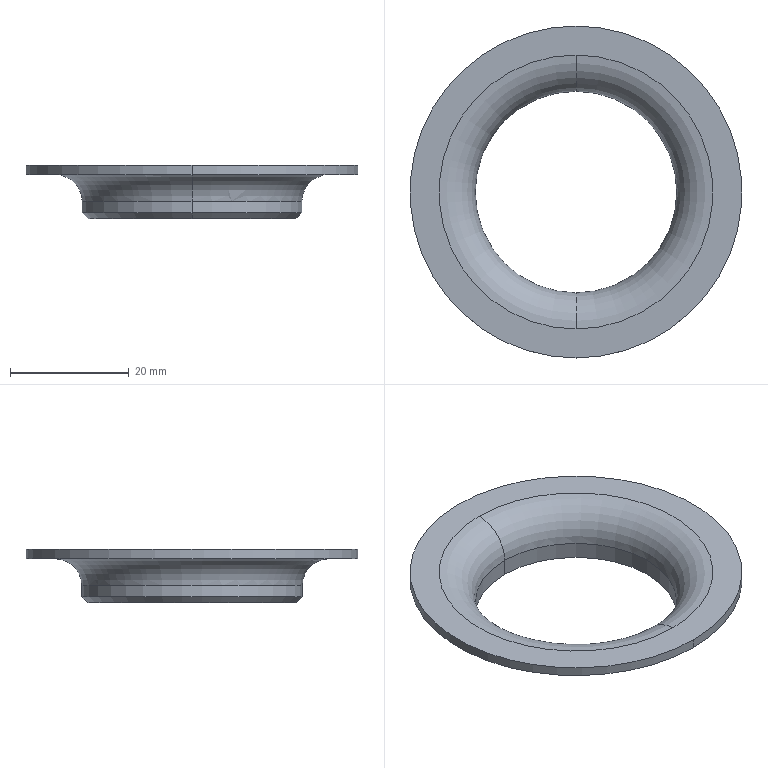Part | STEP file | YLG_9_1_1_1 | 1 solid | 15 faces | box 56 x 56 x 9 mm | volume 3369 mm3 | cylinder 6 | torus 4 | plane 3 | cone 2 | commonest cylinder face diameters 34 x2 37.2 x2 56 x2
STEP:
#1=CARTESIAN_POINT('',(0.,0.,0.));
#2=DIRECTION('',(0.,0.,1.));
#3=DIRECTION('',(1.,0.,0.));
#4=AXIS2_PLACEMENT_3D('',#1,#2,#3);
#5=CARTESIAN_POINT('',(0.,-17.,-10.));
#6=VERTEX_POINT('',#5);
#7=CARTESIAN_POINT('',(0.,-23.1,-3.9));
#8=VERTEX_POINT('',#7);
#9=CARTESIAN_POINT('',(0.,-23.1,-10.));
#10=DIRECTION('',(1.,0.,0.));
#11=DIRECTION('',(0.,1.,0.));
#12=AXIS2_PLACEMENT_3D('',#9,#10,#11);
#13=CIRCLE('',#12,6.1);
#14=EDGE_CURVE('',#6,#8,#13,.T.);
#15=ORIENTED_EDGE('',*,*,#14,.F.);
#16=CARTESIAN_POINT('',(0.,17.,-10.));
#17=VERTEX_POINT('',#16);
#18=CARTESIAN_POINT('',(0.,0.,-10.));
#19=DIRECTION('',(0.,0.,1.));
#20=DIRECTION('',(0.,-1.,0.));
#21=AXIS2_PLACEMENT_3D('',#18,#19,#20);
#22=CIRCLE('',#21,17.);
#23=EDGE_CURVE('',#6,#17,#22,.T.);
#24=ORIENTED_EDGE('',*,*,#23,.T.);
#25=CARTESIAN_POINT('',(0.,23.1,-3.9));
#26=VERTEX_POINT('',#25);
#27=CARTESIAN_POINT('',(0.,23.1,-10.));
#28=DIRECTION('',(-1.,0.,0.));
#29=DIRECTION('',(0.,-1.,0.));
#30=AXIS2_PLACEMENT_3D('',#27,#28,#29);
#31=CIRCLE('',#30,6.1);
#32=EDGE_CURVE('',#17,#26,#31,.T.);
#33=ORIENTED_EDGE('',*,*,#32,.T.);
#34=CARTESIAN_POINT('',(0.,0.,-3.9));
#35=DIRECTION('',(0.,0.,1.));
#36=DIRECTION('',(0.,-1.,0.));
#37=AXIS2_PLACEMENT_3D('',#34,#35,#36);
#38=CIRCLE('',#37,23.1);
#39=EDGE_CURVE('',#8,#26,#38,.T.);
#40=ORIENTED_EDGE('',*,*,#39,.F.);
#41=EDGE_LOOP('',(#15,#24,#33,#40));
#42=FACE_OUTER_BOUND('',#41,.F.);
#43=CARTESIAN_POINT('',(0.,0.,-10.));
#44=DIRECTION('',(0.,0.,1.));
#45=DIRECTION('',(0.,1.,0.));
#46=AXIS2_PLACEMENT_3D('',#43,#44,#45);
#47=TOROIDAL_SURFACE('',#46,23.1,6.1);
#48=ADVANCED_FACE('',(#42),#47,.T.);
#49=ORIENTED_EDGE('',*,*,#14,.T.);
#50=CARTESIAN_POINT('',(0.,0.,-3.9));
#51=DIRECTION('',(0.,0.,1.));
#52=DIRECTION('',(0.,1.,0.));
#53=AXIS2_PLACEMENT_3D('',#50,#51,#52);
#54=CIRCLE('',#53,23.1);
#55=EDGE_CURVE('',#26,#8,#54,.T.);
#56=ORIENTED_EDGE('',*,*,#55,.F.);
#57=ORIENTED_EDGE('',*,*,#32,.F.);
#58=CARTESIAN_POINT('',(0.,0.,-10.));
#59=DIRECTION('',(0.,0.,1.));
#60=DIRECTION('',(0.,1.,0.));
#61=AXIS2_PLACEMENT_3D('',#58,#59,#60);
#62=CIRCLE('',#61,17.);
#63=EDGE_CURVE('',#17,#6,#62,.T.);
#64=ORIENTED_EDGE('',*,*,#63,.T.);
#65=EDGE_LOOP('',(#49,#56,#57,#64));
#66=FACE_OUTER_BOUND('',#65,.F.);
#67=CARTESIAN_POINT('',(0.,0.,-10.));
#68=DIRECTION('',(0.,0.,1.));
#69=DIRECTION('',(0.,1.,0.));
#70=AXIS2_PLACEMENT_3D('',#67,#68,#69);
#71=TOROIDAL_SURFACE('',#70,23.1,6.1);
#72=ADVANCED_FACE('',(#66),#71,.T.);
#73=CARTESIAN_POINT('',(0.,28.,-3.9));
#74=VERTEX_POINT('',#73);
#75=CARTESIAN_POINT('',(0.,-28.,-3.9));
#76=VERTEX_POINT('',#75);
#77=CARTESIAN_POINT('',(0.,0.,-3.9));
#78=DIRECTION('',(0.,0.,-1.));
#79=DIRECTION('',(0.,1.,0.));
#80=AXIS2_PLACEMENT_3D('',#77,#78,#79);
#81=CIRCLE('',#80,28.);
#82=EDGE_CURVE('',#74,#76,#81,.T.);
#83=ORIENTED_EDGE('',*,*,#82,.T.);
#84=CARTESIAN_POINT('',(0.,0.,-3.9));
#85=DIRECTION('',(0.,0.,-1.));
#86=DIRECTION('',(0.,-1.,0.));
#87=AXIS2_PLACEMENT_3D('',#84,#85,#86);
#88=CIRCLE('',#87,28.);
#89=EDGE_CURVE('',#76,#74,#88,.T.);
#90=ORIENTED_EDGE('',*,*,#89,.T.);
#91=EDGE_LOOP('',(#83,#90));
#92=FACE_OUTER_BOUND('',#91,.F.);
#93=ORIENTED_EDGE('',*,*,#55,.T.);
#94=ORIENTED_EDGE('',*,*,#39,.T.);
#95=EDGE_LOOP('',(#93,#94));
#96=FACE_BOUND('',#95,.F.);
#97=CARTESIAN_POINT('',(0.,0.,-3.9));
#98=DIRECTION('',(0.,0.,1.));
#99=DIRECTION('',(0.,1.,0.));
#100=AXIS2_PLACEMENT_3D('',#97,#98,#99);
#101=PLANE('',#100);
#102=ADVANCED_FACE('',(#92,#96),#101,.T.);
#103=CARTESIAN_POINT('',(0.,-28.,-5.5));
#104=VERTEX_POINT('',#103);
#105=CARTESIAN_POINT('',(0.,-28.,-3.9));
#106=DIRECTION('',(0.,0.,-1.));
#107=VECTOR('',#106,1.6);
#108=LINE('',#105,#107);
#109=EDGE_CURVE('',#76,#104,#108,.T.);
#110=ORIENTED_EDGE('',*,*,#109,.F.);
#111=ORIENTED_EDGE('',*,*,#82,.F.);
#112=CARTESIAN_POINT('',(0.,28.,-5.5));
#113=VERTEX_POINT('',#112);
#114=CARTESIAN_POINT('',(0.,28.,-3.9));
#115=DIRECTION('',(0.,0.,-1.));
#116=VECTOR('',#115,1.6);
#117=LINE('',#114,#116);
#118=EDGE_CURVE('',#74,#113,#117,.T.);
#119=ORIENTED_EDGE('',*,*,#118,.T.);
#120=CARTESIAN_POINT('',(0.,0.,-5.5));
#121=DIRECTION('',(0.,0.,1.));
#122=DIRECTION('',(0.,-1.,0.));
#123=AXIS2_PLACEMENT_3D('',#120,#121,#122);
#124=CIRCLE('',#123,28.);
#125=EDGE_CURVE('',#104,#113,#124,.T.);
#126=ORIENTED_EDGE('',*,*,#125,.F.);
#127=EDGE_LOOP('',(#110,#111,#119,#126));
#128=FACE_OUTER_BOUND('',#127,.F.);
#129=CARTESIAN_POINT('',(0.,0.,0.));
#130=DIRECTION('',(0.,0.,1.));
#131=DIRECTION('',(0.,1.,0.));
#132=AXIS2_PLACEMENT_3D('',#129,#130,#131);
#133=CYLINDRICAL_SURFACE('',#132,28.);
#134=ADVANCED_FACE('',(#128),#133,.T.);
#135=ORIENTED_EDGE('',*,*,#109,.T.);
#136=CARTESIAN_POINT('',(0.,0.,-5.5));
#137=DIRECTION('',(0.,0.,1.));
#138=DIRECTION('',(0.,1.,0.));
#139=AXIS2_PLACEMENT_3D('',#136,#137,#138);
#140=CIRCLE('',#139,28.);
#141=EDGE_CURVE('',#113,#104,#140,.T.);
#142=ORIENTED_EDGE('',*,*,#141,.F.);
#143=ORIENTED_EDGE('',*,*,#118,.F.);
#144=ORIENTED_EDGE('',*,*,#89,.F.);
#145=EDGE_LOOP('',(#135,#142,#143,#144));
#146=FACE_OUTER_BOUND('',#145,.F.);
#147=CARTESIAN_POINT('',(0.,0.,0.));
#148=DIRECTION('',(0.,0.,1.));
#149=DIRECTION('',(0.,1.,0.));
#150=AXIS2_PLACEMENT_3D('',#147,#148,#149);
#151=CYLINDRICAL_SURFACE('',#150,28.);
#152=ADVANCED_FACE('',(#146),#151,.T.);
#153=ORIENTED_EDGE('',*,*,#141,.T.);
#154=ORIENTED_EDGE('',*,*,#125,.T.);
#155=EDGE_LOOP('',(#153,#154));
#156=FACE_OUTER_BOUND('',#155,.F.);
#157=CARTESIAN_POINT('',(0.,23.1,-5.5));
#158=VERTEX_POINT('',#157);
#159=CARTESIAN_POINT('',(0.,-23.1,-5.5));
#160=VERTEX_POINT('',#159);
#161=CARTESIAN_POINT('',(0.,0.,-5.5));
#162=DIRECTION('',(0.,0.,-1.));
#163=DIRECTION('',(0.,1.,0.));
#164=AXIS2_PLACEMENT_3D('',#161,#162,#163);
#165=CIRCLE('',#164,23.1);
#166=EDGE_CURVE('',#158,#160,#165,.T.);
#167=ORIENTED_EDGE('',*,*,#166,.T.);
#168=CARTESIAN_POINT('',(0.,0.,-5.5));
#169=DIRECTION('',(0.,0.,-1.));
#170=DIRECTION('',(0.,-1.,0.));
#171=AXIS2_PLACEMENT_3D('',#168,#169,#170);
#172=CIRCLE('',#171,23.1);
#173=EDGE_CURVE('',#160,#158,#172,.T.);
#174=ORIENTED_EDGE('',*,*,#173,.T.);
#175=EDGE_LOOP('',(#167,#174));
#176=FACE_BOUND('',#175,.F.);
#177=CARTESIAN_POINT('',(0.,0.,-5.5));
#178=DIRECTION('',(0.,0.,1.));
#179=DIRECTION('',(0.,1.,0.));
#180=AXIS2_PLACEMENT_3D('',#177,#178,#179);
#181=PLANE('',#180);
#182=ADVANCED_FACE('',(#156,#176),#181,.F.);
#183=CARTESIAN_POINT('',(0.,-18.6,-10.));
#184=VERTEX_POINT('',#183);
#185=CARTESIAN_POINT('',(0.,-23.1,-10.));
#186=DIRECTION('',(-1.,0.,0.));
#187=DIRECTION('',(0.,0.,1.));
#188=AXIS2_PLACEMENT_3D('',#185,#186,#187);
#189=CIRCLE('',#188,4.5);
#190=EDGE_CURVE('',#160,#184,#189,.T.);
#191=ORIENTED_EDGE('',*,*,#190,.F.);
#192=ORIENTED_EDGE('',*,*,#166,.F.);
#193=CARTESIAN_POINT('',(0.,18.6,-10.));
#194=VERTEX_POINT('',#193);
#195=CARTESIAN_POINT('',(0.,23.1,-10.));
#196=DIRECTION('',(1.,0.,0.));
#197=DIRECTION('',(0.,0.,1.));
#198=AXIS2_PLACEMENT_3D('',#195,#196,#197);
#199=CIRCLE('',#198,4.5);
#200=EDGE_CURVE('',#158,#194,#199,.T.);
#201=ORIENTED_EDGE('',*,*,#200,.T.);
#202=CARTESIAN_POINT('',(0.,0.,-10.));
#203=DIRECTION('',(0.,0.,-1.));
#204=DIRECTION('',(0.,1.,0.));
#205=AXIS2_PLACEMENT_3D('',#202,#203,#204);
#206=CIRCLE('',#205,18.6);
#207=EDGE_CURVE('',#194,#184,#206,.T.);
#208=ORIENTED_EDGE('',*,*,#207,.T.);
#209=EDGE_LOOP('',(#191,#192,#201,#208));
#210=FACE_OUTER_BOUND('',#209,.F.);
#211=CARTESIAN_POINT('',(0.,0.,-10.));
#212=DIRECTION('',(0.,0.,1.));
#213=DIRECTION('',(0.,1.,0.));
#214=AXIS2_PLACEMENT_3D('',#211,#212,#213);
#215=TOROIDAL_SURFACE('',#214,23.1,4.5);
#216=ADVANCED_FACE('',(#210),#215,.F.);
#217=ORIENTED_EDGE('',*,*,#190,.T.);
#218=CARTESIAN_POINT('',(0.,0.,-10.));
#219=DIRECTION('',(0.,0.,-1.));
#220=DIRECTION('',(0.,-1.,0.));
#221=AXIS2_PLACEMENT_3D('',#218,#219,#220);
#222=CIRCLE('',#221,18.6);
#223=EDGE_CURVE('',#184,#194,#222,.T.);
#224=ORIENTED_EDGE('',*,*,#223,.T.);
#225=ORIENTED_EDGE('',*,*,#200,.F.);
#226=ORIENTED_EDGE('',*,*,#173,.F.);
#227=EDGE_LOOP('',(#217,#224,#225,#226));
#228=FACE_OUTER_BOUND('',#227,.F.);
#229=CARTESIAN_POINT('',(0.,0.,-10.));
#230=DIRECTION('',(0.,0.,1.));
#231=DIRECTION('',(0.,1.,0.));
#232=AXIS2_PLACEMENT_3D('',#229,#230,#231);
#233=TOROIDAL_SURFACE('',#232,23.1,4.5);
#234=ADVANCED_FACE('',(#228),#233,.F.);
#235=CARTESIAN_POINT('',(0.,18.6,-11.9));
#236=VERTEX_POINT('',#235);
#237=CARTESIAN_POINT('',(0.,-18.6,-11.9));
#238=VERTEX_POINT('',#237);
#239=CARTESIAN_POINT('',(0.,0.,-11.9));
#240=DIRECTION('',(0.,0.,1.));
#241=DIRECTION('',(0.,1.,0.));
#242=AXIS2_PLACEMENT_3D('',#239,#240,#241);
#243=CIRCLE('',#242,18.6);
#244=EDGE_CURVE('',#236,#238,#243,.T.);
#245=ORIENTED_EDGE('',*,*,#244,.F.);
#246=CARTESIAN_POINT('',(0.,18.6,-10.));
#247=DIRECTION('',(0.,0.,-1.));
#248=VECTOR('',#247,1.9);
#249=LINE('',#246,#248);
#250=EDGE_CURVE('',#194,#236,#249,.T.);
#251=ORIENTED_EDGE('',*,*,#250,.F.);
#252=ORIENTED_EDGE('',*,*,#223,.F.);
#253=CARTESIAN_POINT('',(0.,-18.6,-10.));
#254=DIRECTION('',(0.,0.,-1.));
#255=VECTOR('',#254,1.9);
#256=LINE('',#253,#255);
#257=EDGE_CURVE('',#184,#238,#256,.T.);
#258=ORIENTED_EDGE('',*,*,#257,.T.);
#259=EDGE_LOOP('',(#245,#251,#252,#258));
#260=FACE_OUTER_BOUND('',#259,.F.);
#261=CARTESIAN_POINT('',(0.,0.,0.));
#262=DIRECTION('',(0.,0.,1.));
#263=DIRECTION('',(0.,1.,0.));
#264=AXIS2_PLACEMENT_3D('',#261,#262,#263);
#265=CYLINDRICAL_SURFACE('',#264,18.6);
#266=ADVANCED_FACE('',(#260),#265,.T.);
#267=CARTESIAN_POINT('',(0.,17.6,-12.9));
#268=VERTEX_POINT('',#267);
#269=CARTESIAN_POINT('',(0.,-17.6,-12.9));
#270=VERTEX_POINT('',#269);
#271=CARTESIAN_POINT('',(0.,0.,-12.9));
#272=DIRECTION('',(0.,0.,1.));
#273=DIRECTION('',(0.,1.,0.));
#274=AXIS2_PLACEMENT_3D('',#271,#272,#273);
#275=CIRCLE('',#274,17.6);
#276=EDGE_CURVE('',#268,#270,#275,.T.);
#277=ORIENTED_EDGE('',*,*,#276,.F.);
#278=CARTESIAN_POINT('',(0.,17.6,-12.9));
#279=DIRECTION('',(0.,0.7071,0.7071));
#280=VECTOR('',#279,1.414);
#281=LINE('',#278,#280);
#282=EDGE_CURVE('',#268,#236,#281,.T.);
#283=ORIENTED_EDGE('',*,*,#282,.T.);
#284=ORIENTED_EDGE('',*,*,#244,.T.);
#285=CARTESIAN_POINT('',(0.,-17.6,-12.9));
#286=DIRECTION('',(0.,-0.7071,0.7071));
#287=VECTOR('',#286,1.414);
#288=LINE('',#285,#287);
#289=EDGE_CURVE('',#270,#238,#288,.T.);
#290=ORIENTED_EDGE('',*,*,#289,.F.);
#291=EDGE_LOOP('',(#277,#283,#284,#290));
#292=FACE_OUTER_BOUND('',#291,.F.);
#293=CARTESIAN_POINT('',(0.,0.,-12.4));
#294=DIRECTION('',(0.,0.,1.));
#295=DIRECTION('',(0.,-1.,0.));
#296=AXIS2_PLACEMENT_3D('',#293,#294,#295);
#297=CONICAL_SURFACE('',#296,18.1,45.);
#298=ADVANCED_FACE('',(#292),#297,.T.);
#299=CARTESIAN_POINT('',(0.,0.,-12.9));
#300=DIRECTION('',(0.,0.,1.));
#301=DIRECTION('',(0.,-1.,0.));
#302=AXIS2_PLACEMENT_3D('',#299,#300,#301);
#303=CIRCLE('',#302,17.6);
#304=EDGE_CURVE('',#270,#268,#303,.T.);
#305=ORIENTED_EDGE('',*,*,#304,.T.);
#306=ORIENTED_EDGE('',*,*,#276,.T.);
#307=EDGE_LOOP('',(#305,#306));
#308=FACE_OUTER_BOUND('',#307,.F.);
#309=CARTESIAN_POINT('',(0.,17.,-12.9));
#310=VERTEX_POINT('',#309);
#311=CARTESIAN_POINT('',(0.,-17.,-12.9));
#312=VERTEX_POINT('',#311);
#313=CARTESIAN_POINT('',(0.,0.,-12.9));
#314=DIRECTION('',(0.,0.,-1.));
#315=DIRECTION('',(0.,1.,0.));
#316=AXIS2_PLACEMENT_3D('',#313,#314,#315);
#317=CIRCLE('',#316,17.);
#318=EDGE_CURVE('',#310,#312,#317,.T.);
#319=ORIENTED_EDGE('',*,*,#318,.T.);
#320=CARTESIAN_POINT('',(0.,0.,-12.9));
#321=DIRECTION('',(0.,0.,-1.));
#322=DIRECTION('',(0.,-1.,0.));
#323=AXIS2_PLACEMENT_3D('',#320,#321,#322);
#324=CIRCLE('',#323,17.);
#325=EDGE_CURVE('',#312,#310,#324,.T.);
#326=ORIENTED_EDGE('',*,*,#325,.T.);
#327=EDGE_LOOP('',(#319,#326));
#328=FACE_BOUND('',#327,.F.);
#329=CARTESIAN_POINT('',(0.,0.,-12.9));
#330=DIRECTION('',(0.,0.,1.));
#331=DIRECTION('',(0.,1.,0.));
#332=AXIS2_PLACEMENT_3D('',#329,#330,#331);
#333=PLANE('',#332);
#334=ADVANCED_FACE('',(#308,#328),#333,.F.);
#335=ORIENTED_EDGE('',*,*,#304,.F.);
#336=ORIENTED_EDGE('',*,*,#289,.T.);
#337=CARTESIAN_POINT('',(0.,0.,-11.9));
#338=DIRECTION('',(0.,0.,1.));
#339=DIRECTION('',(0.,-1.,0.));
#340=AXIS2_PLACEMENT_3D('',#337,#338,#339);
#341=CIRCLE('',#340,18.6);
#342=EDGE_CURVE('',#238,#236,#341,.T.);
#343=ORIENTED_EDGE('',*,*,#342,.T.);
#344=ORIENTED_EDGE('',*,*,#282,.F.);
#345=EDGE_LOOP('',(#335,#336,#343,#344));
#346=FACE_OUTER_BOUND('',#345,.F.);
#347=CARTESIAN_POINT('',(0.,0.,-12.4));
#348=DIRECTION('',(0.,0.,1.));
#349=DIRECTION('',(0.,-1.,0.));
#350=AXIS2_PLACEMENT_3D('',#347,#348,#349);
#351=CONICAL_SURFACE('',#350,18.1,45.);
#352=ADVANCED_FACE('',(#346),#351,.T.);
#353=ORIENTED_EDGE('',*,*,#342,.F.);
#354=ORIENTED_EDGE('',*,*,#257,.F.);
#355=ORIENTED_EDGE('',*,*,#207,.F.);
#356=ORIENTED_EDGE('',*,*,#250,.T.);
#357=EDGE_LOOP('',(#353,#354,#355,#356));
#358=FACE_OUTER_BOUND('',#357,.F.);
#359=CARTESIAN_POINT('',(0.,0.,0.));
#360=DIRECTION('',(0.,0.,1.));
#361=DIRECTION('',(0.,1.,0.));
#362=AXIS2_PLACEMENT_3D('',#359,#360,#361);
#363=CYLINDRICAL_SURFACE('',#362,18.6);
#364=ADVANCED_FACE('',(#358),#363,.T.);
#365=CARTESIAN_POINT('',(0.,-17.,-12.9));
#366=DIRECTION('',(0.,0.,1.));
#367=VECTOR('',#366,2.9);
#368=LINE('',#365,#367);
#369=EDGE_CURVE('',#312,#6,#368,.T.);
#370=ORIENTED_EDGE('',*,*,#369,.F.);
#371=ORIENTED_EDGE('',*,*,#318,.F.);
#372=CARTESIAN_POINT('',(0.,17.,-12.9));
#373=DIRECTION('',(0.,0.,1.));
#374=VECTOR('',#373,2.9);
#375=LINE('',#372,#374);
#376=EDGE_CURVE('',#310,#17,#375,.T.);
#377=ORIENTED_EDGE('',*,*,#376,.T.);
#378=ORIENTED_EDGE('',*,*,#23,.F.);
#379=EDGE_LOOP('',(#370,#371,#377,#378));
#380=FACE_OUTER_BOUND('',#379,.F.);
#381=CARTESIAN_POINT('',(0.,0.,0.));
#382=DIRECTION('',(0.,0.,1.));
#383=DIRECTION('',(0.,1.,0.));
#384=AXIS2_PLACEMENT_3D('',#381,#382,#383);
#385=CYLINDRICAL_SURFACE('',#384,17.);
#386=ADVANCED_FACE('',(#380),#385,.F.);
#387=ORIENTED_EDGE('',*,*,#369,.T.);
#388=ORIENTED_EDGE('',*,*,#63,.F.);
#389=ORIENTED_EDGE('',*,*,#376,.F.);
#390=ORIENTED_EDGE('',*,*,#325,.F.);
#391=EDGE_LOOP('',(#387,#388,#389,#390));
#392=FACE_OUTER_BOUND('',#391,.F.);
#393=CARTESIAN_POINT('',(0.,0.,0.));
#394=DIRECTION('',(0.,0.,1.));
#395=DIRECTION('',(0.,1.,0.));
#396=AXIS2_PLACEMENT_3D('',#393,#394,#395);
#397=CYLINDRICAL_SURFACE('',#396,17.);
#398=ADVANCED_FACE('',(#392),#397,.F.);
#399=CLOSED_SHELL('',(#48,#72,#102,#134,#152,#182,#216,#234,#266,#298,#334,#352,#364,#386,#398));
#400=MANIFOLD_SOLID_BREP('',#399);
#401=(LENGTH_UNIT()NAMED_UNIT(*)SI_UNIT(.MILLI.,.METRE.));
#402=UNCERTAINTY_MEASURE_WITH_UNIT(LENGTH_MEASURE(0.007973),#401,'','');
#403=(NAMED_UNIT(*)PLANE_ANGLE_UNIT()SI_UNIT($,.RADIAN.));
#404=PLANE_ANGLE_MEASURE_WITH_UNIT(PLANE_ANGLE_MEASURE(0.01745),#403);
#405=(CONVERSION_BASED_UNIT('DEGREE',#404)NAMED_UNIT(*)PLANE_ANGLE_UNIT());
#406=(NAMED_UNIT(*)SI_UNIT($,.STERADIAN.)SOLID_ANGLE_UNIT());
#407=(GEOMETRIC_REPRESENTATION_CONTEXT(3)GLOBAL_UNCERTAINTY_ASSIGNED_CONTEXT((#402))GLOBAL_UNIT_ASSIGNED_CONTEXT((#401,#405,#406))REPRESENTATION_CONTEXT('',''));
#408=ADVANCED_BREP_SHAPE_REPRESENTATION('',(#4,#400),#407);